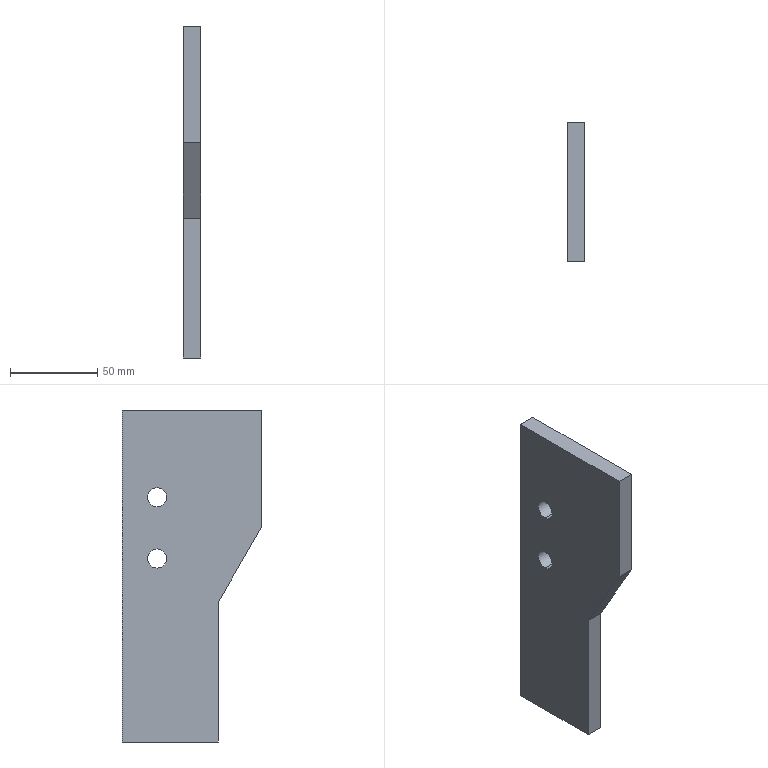Part | STEP file | VD-SYL0380DJ1006_1_5-3_VD-SYL03 | 1 solid | 12 faces | box 10 x 80 x 190 mm | volume 124687 mm3 | plane 8 | cylinder 4 | commonest cylinder face diameters 11 x4
STEP:
#1=CARTESIAN_POINT('',(0.,-20.,-90.5));
#2=VERTEX_POINT('',#1);
#3=CARTESIAN_POINT('',(10.,-20.,-90.5));
#4=VERTEX_POINT('',#3);
#5=CARTESIAN_POINT('',(0.,-20.,-90.5));
#6=DIRECTION('',(1.,0.,0.));
#7=VECTOR('',#6,1000.);
#8=LINE('',#5,#7);
#9=EDGE_CURVE('',#2,#4,#8,.T.);
#10=ORIENTED_EDGE('',*,*,#9,.F.);
#11=CARTESIAN_POINT('',(0.,-20.,-79.5));
#12=VERTEX_POINT('',#11);
#13=CARTESIAN_POINT('',(0.,-20.,-85.));
#14=DIRECTION('',(1.,0.,0.));
#15=DIRECTION('',(0.,0.,1.));
#16=AXIS2_PLACEMENT_3D('',#13,#14,#15);
#17=CIRCLE('',#16,5.5);
#18=EDGE_CURVE('',#12,#2,#17,.T.);
#19=ORIENTED_EDGE('',*,*,#18,.F.);
#20=CARTESIAN_POINT('',(10.,-20.,-79.5));
#21=VERTEX_POINT('',#20);
#22=CARTESIAN_POINT('',(0.,-20.,-79.5));
#23=DIRECTION('',(1.,0.,0.));
#24=VECTOR('',#23,1000.);
#25=LINE('',#22,#24);
#26=EDGE_CURVE('',#12,#21,#25,.T.);
#27=ORIENTED_EDGE('',*,*,#26,.T.);
#28=CARTESIAN_POINT('',(10.,-20.,-85.));
#29=DIRECTION('',(-1.,0.,0.));
#30=DIRECTION('',(0.,0.,-1.));
#31=AXIS2_PLACEMENT_3D('',#28,#29,#30);
#32=CIRCLE('',#31,5.5);
#33=EDGE_CURVE('',#4,#21,#32,.T.);
#34=ORIENTED_EDGE('',*,*,#33,.F.);
#35=EDGE_LOOP('',(#10,#19,#27,#34));
#36=FACE_OUTER_BOUND('',#35,.T.);
#37=CARTESIAN_POINT('',(0.,-20.,-85.));
#38=DIRECTION('',(-1.,0.,0.));
#39=DIRECTION('',(0.,0.,1.));
#40=AXIS2_PLACEMENT_3D('',#37,#38,#39);
#41=CYLINDRICAL_SURFACE('',#40,5.5);
#42=ADVANCED_FACE('',(#36),#41,.F.);
#43=CARTESIAN_POINT('',(10.,-20.,-85.));
#44=DIRECTION('',(-1.,0.,0.));
#45=DIRECTION('',(0.,0.,1.));
#46=AXIS2_PLACEMENT_3D('',#43,#44,#45);
#47=CIRCLE('',#46,5.5);
#48=EDGE_CURVE('',#21,#4,#47,.T.);
#49=ORIENTED_EDGE('',*,*,#48,.F.);
#50=ORIENTED_EDGE('',*,*,#26,.F.);
#51=CARTESIAN_POINT('',(0.,-20.,-85.));
#52=DIRECTION('',(1.,0.,0.));
#53=DIRECTION('',(0.,0.,-1.));
#54=AXIS2_PLACEMENT_3D('',#51,#52,#53);
#55=CIRCLE('',#54,5.5);
#56=EDGE_CURVE('',#2,#12,#55,.T.);
#57=ORIENTED_EDGE('',*,*,#56,.F.);
#58=ORIENTED_EDGE('',*,*,#9,.T.);
#59=EDGE_LOOP('',(#49,#50,#57,#58));
#60=FACE_OUTER_BOUND('',#59,.T.);
#61=CARTESIAN_POINT('',(0.,-20.,-85.));
#62=DIRECTION('',(-1.,0.,0.));
#63=DIRECTION('',(0.,0.,1.));
#64=AXIS2_PLACEMENT_3D('',#61,#62,#63);
#65=CYLINDRICAL_SURFACE('',#64,5.5);
#66=ADVANCED_FACE('',(#60),#65,.F.);
#67=CARTESIAN_POINT('',(0.,-20.,-55.5));
#68=VERTEX_POINT('',#67);
#69=CARTESIAN_POINT('',(10.,-20.,-55.5));
#70=VERTEX_POINT('',#69);
#71=CARTESIAN_POINT('',(0.,-20.,-55.5));
#72=DIRECTION('',(1.,0.,0.));
#73=VECTOR('',#72,1000.);
#74=LINE('',#71,#73);
#75=EDGE_CURVE('',#68,#70,#74,.T.);
#76=ORIENTED_EDGE('',*,*,#75,.F.);
#77=CARTESIAN_POINT('',(0.,-20.,-44.5));
#78=VERTEX_POINT('',#77);
#79=CARTESIAN_POINT('',(0.,-20.,-50.));
#80=DIRECTION('',(1.,0.,0.));
#81=DIRECTION('',(0.,0.,1.));
#82=AXIS2_PLACEMENT_3D('',#79,#80,#81);
#83=CIRCLE('',#82,5.5);
#84=EDGE_CURVE('',#78,#68,#83,.T.);
#85=ORIENTED_EDGE('',*,*,#84,.F.);
#86=CARTESIAN_POINT('',(10.,-20.,-44.5));
#87=VERTEX_POINT('',#86);
#88=CARTESIAN_POINT('',(0.,-20.,-44.5));
#89=DIRECTION('',(1.,0.,0.));
#90=VECTOR('',#89,1000.);
#91=LINE('',#88,#90);
#92=EDGE_CURVE('',#78,#87,#91,.T.);
#93=ORIENTED_EDGE('',*,*,#92,.T.);
#94=CARTESIAN_POINT('',(10.,-20.,-50.));
#95=DIRECTION('',(-1.,0.,0.));
#96=DIRECTION('',(0.,0.,-1.));
#97=AXIS2_PLACEMENT_3D('',#94,#95,#96);
#98=CIRCLE('',#97,5.5);
#99=EDGE_CURVE('',#70,#87,#98,.T.);
#100=ORIENTED_EDGE('',*,*,#99,.F.);
#101=EDGE_LOOP('',(#76,#85,#93,#100));
#102=FACE_OUTER_BOUND('',#101,.T.);
#103=CARTESIAN_POINT('',(0.,-20.,-50.));
#104=DIRECTION('',(-1.,0.,0.));
#105=DIRECTION('',(0.,0.,1.));
#106=AXIS2_PLACEMENT_3D('',#103,#104,#105);
#107=CYLINDRICAL_SURFACE('',#106,5.5);
#108=ADVANCED_FACE('',(#102),#107,.F.);
#109=CARTESIAN_POINT('',(10.,-20.,-50.));
#110=DIRECTION('',(-1.,0.,0.));
#111=DIRECTION('',(0.,0.,1.));
#112=AXIS2_PLACEMENT_3D('',#109,#110,#111);
#113=CIRCLE('',#112,5.5);
#114=EDGE_CURVE('',#87,#70,#113,.T.);
#115=ORIENTED_EDGE('',*,*,#114,.F.);
#116=ORIENTED_EDGE('',*,*,#92,.F.);
#117=CARTESIAN_POINT('',(0.,-20.,-50.));
#118=DIRECTION('',(1.,0.,0.));
#119=DIRECTION('',(0.,0.,-1.));
#120=AXIS2_PLACEMENT_3D('',#117,#118,#119);
#121=CIRCLE('',#120,5.5);
#122=EDGE_CURVE('',#68,#78,#121,.T.);
#123=ORIENTED_EDGE('',*,*,#122,.F.);
#124=ORIENTED_EDGE('',*,*,#75,.T.);
#125=EDGE_LOOP('',(#115,#116,#123,#124));
#126=FACE_OUTER_BOUND('',#125,.T.);
#127=CARTESIAN_POINT('',(0.,-20.,-50.));
#128=DIRECTION('',(-1.,0.,0.));
#129=DIRECTION('',(0.,0.,1.));
#130=AXIS2_PLACEMENT_3D('',#127,#128,#129);
#131=CYLINDRICAL_SURFACE('',#130,5.5);
#132=ADVANCED_FACE('',(#126),#131,.F.);
#133=CARTESIAN_POINT('',(10.,-55.,-110.));
#134=VERTEX_POINT('',#133);
#135=CARTESIAN_POINT('',(10.,-55.,-190.));
#136=VERTEX_POINT('',#135);
#137=CARTESIAN_POINT('',(10.,-55.,-110.));
#138=DIRECTION('',(0.,0.,-1.));
#139=VECTOR('',#138,1000.);
#140=LINE('',#137,#139);
#141=EDGE_CURVE('',#134,#136,#140,.T.);
#142=ORIENTED_EDGE('',*,*,#141,.F.);
#143=CARTESIAN_POINT('',(0.,-55.,-110.));
#144=VERTEX_POINT('',#143);
#145=CARTESIAN_POINT('',(10.,-55.,-110.));
#146=DIRECTION('',(-1.,0.,0.));
#147=VECTOR('',#146,1000.);
#148=LINE('',#145,#147);
#149=EDGE_CURVE('',#134,#144,#148,.T.);
#150=ORIENTED_EDGE('',*,*,#149,.T.);
#151=CARTESIAN_POINT('',(0.,-55.,-190.));
#152=VERTEX_POINT('',#151);
#153=CARTESIAN_POINT('',(0.,-55.,-190.));
#154=DIRECTION('',(0.,0.,1.));
#155=VECTOR('',#154,1000.);
#156=LINE('',#153,#155);
#157=EDGE_CURVE('',#152,#144,#156,.T.);
#158=ORIENTED_EDGE('',*,*,#157,.F.);
#159=CARTESIAN_POINT('',(0.,-55.,-190.));
#160=DIRECTION('',(1.,0.,0.));
#161=VECTOR('',#160,1000.);
#162=LINE('',#159,#161);
#163=EDGE_CURVE('',#152,#136,#162,.T.);
#164=ORIENTED_EDGE('',*,*,#163,.T.);
#165=EDGE_LOOP('',(#142,#150,#158,#164));
#166=FACE_OUTER_BOUND('',#165,.T.);
#167=CARTESIAN_POINT('',(0.,-55.,-110.));
#168=DIRECTION('',(0.,-1.,0.));
#169=DIRECTION('',(0.,0.,-1.));
#170=AXIS2_PLACEMENT_3D('',#167,#168,#169);
#171=PLANE('',#170);
#172=ADVANCED_FACE('',(#166),#171,.T.);
#173=ORIENTED_EDGE('',*,*,#33,.T.);
#174=ORIENTED_EDGE('',*,*,#48,.T.);
#175=EDGE_LOOP('',(#173,#174));
#176=FACE_BOUND('',#175,.T.);
#177=ORIENTED_EDGE('',*,*,#99,.T.);
#178=ORIENTED_EDGE('',*,*,#114,.T.);
#179=EDGE_LOOP('',(#177,#178));
#180=FACE_BOUND('',#179,.T.);
#181=CARTESIAN_POINT('',(10.,0.,-190.));
#182=VERTEX_POINT('',#181);
#183=CARTESIAN_POINT('',(10.,0.,0.));
#184=VERTEX_POINT('',#183);
#185=CARTESIAN_POINT('',(10.,0.,-190.));
#186=DIRECTION('',(0.,0.,1.));
#187=VECTOR('',#186,1000.);
#188=LINE('',#185,#187);
#189=EDGE_CURVE('',#182,#184,#188,.T.);
#190=ORIENTED_EDGE('',*,*,#189,.T.);
#191=CARTESIAN_POINT('',(10.,-80.,0.));
#192=VERTEX_POINT('',#191);
#193=CARTESIAN_POINT('',(10.,0.,0.));
#194=DIRECTION('',(0.,-1.,0.));
#195=VECTOR('',#194,1000.);
#196=LINE('',#193,#195);
#197=EDGE_CURVE('',#184,#192,#196,.T.);
#198=ORIENTED_EDGE('',*,*,#197,.T.);
#199=CARTESIAN_POINT('',(10.,-80.,-66.699));
#200=VERTEX_POINT('',#199);
#201=CARTESIAN_POINT('',(10.,-80.,0.));
#202=DIRECTION('',(0.,0.,-1.));
#203=VECTOR('',#202,1000.);
#204=LINE('',#201,#203);
#205=EDGE_CURVE('',#192,#200,#204,.T.);
#206=ORIENTED_EDGE('',*,*,#205,.T.);
#207=CARTESIAN_POINT('',(10.,-80.,-66.699));
#208=DIRECTION('',(0.,0.5,-0.866));
#209=VECTOR('',#208,1000.);
#210=LINE('',#207,#209);
#211=EDGE_CURVE('',#200,#134,#210,.T.);
#212=ORIENTED_EDGE('',*,*,#211,.T.);
#213=ORIENTED_EDGE('',*,*,#141,.T.);
#214=CARTESIAN_POINT('',(10.,-55.,-190.));
#215=DIRECTION('',(0.,1.,0.));
#216=VECTOR('',#215,1000.);
#217=LINE('',#214,#216);
#218=EDGE_CURVE('',#136,#182,#217,.T.);
#219=ORIENTED_EDGE('',*,*,#218,.T.);
#220=EDGE_LOOP('',(#190,#198,#206,#212,#213,#219));
#221=FACE_OUTER_BOUND('',#220,.T.);
#222=CARTESIAN_POINT('',(10.,0.,0.));
#223=DIRECTION('',(1.,0.,0.));
#224=DIRECTION('',(0.,1.,0.));
#225=AXIS2_PLACEMENT_3D('',#222,#223,#224);
#226=PLANE('',#225);
#227=ADVANCED_FACE('',(#176,#180,#221),#226,.T.);
#228=CARTESIAN_POINT('',(0.,-80.,-66.699));
#229=VERTEX_POINT('',#228);
#230=CARTESIAN_POINT('',(0.,-55.,-110.));
#231=DIRECTION('',(0.,-0.5,0.866));
#232=VECTOR('',#231,1000.);
#233=LINE('',#230,#232);
#234=EDGE_CURVE('',#144,#229,#233,.T.);
#235=ORIENTED_EDGE('',*,*,#234,.F.);
#236=ORIENTED_EDGE('',*,*,#149,.F.);
#237=ORIENTED_EDGE('',*,*,#211,.F.);
#238=CARTESIAN_POINT('',(0.,-80.,-66.699));
#239=DIRECTION('',(1.,0.,0.));
#240=VECTOR('',#239,1000.);
#241=LINE('',#238,#240);
#242=EDGE_CURVE('',#229,#200,#241,.T.);
#243=ORIENTED_EDGE('',*,*,#242,.F.);
#244=EDGE_LOOP('',(#235,#236,#237,#243));
#245=FACE_OUTER_BOUND('',#244,.T.);
#246=CARTESIAN_POINT('',(0.,-80.,-66.699));
#247=DIRECTION('',(0.,-0.866,-0.5));
#248=DIRECTION('',(0.,0.5,-0.866));
#249=AXIS2_PLACEMENT_3D('',#246,#247,#248);
#250=PLANE('',#249);
#251=ADVANCED_FACE('',(#245),#250,.T.);
#252=ORIENTED_EDGE('',*,*,#18,.T.);
#253=ORIENTED_EDGE('',*,*,#56,.T.);
#254=EDGE_LOOP('',(#252,#253));
#255=FACE_BOUND('',#254,.T.);
#256=ORIENTED_EDGE('',*,*,#84,.T.);
#257=ORIENTED_EDGE('',*,*,#122,.T.);
#258=EDGE_LOOP('',(#256,#257));
#259=FACE_BOUND('',#258,.T.);
#260=CARTESIAN_POINT('',(0.,-80.,0.));
#261=VERTEX_POINT('',#260);
#262=CARTESIAN_POINT('',(0.,0.,0.));
#263=VERTEX_POINT('',#262);
#264=CARTESIAN_POINT('',(0.,-80.,0.));
#265=DIRECTION('',(0.,1.,0.));
#266=VECTOR('',#265,1000.);
#267=LINE('',#264,#266);
#268=EDGE_CURVE('',#261,#263,#267,.T.);
#269=ORIENTED_EDGE('',*,*,#268,.T.);
#270=CARTESIAN_POINT('',(0.,0.,-190.));
#271=VERTEX_POINT('',#270);
#272=CARTESIAN_POINT('',(0.,0.,0.));
#273=DIRECTION('',(0.,0.,-1.));
#274=VECTOR('',#273,1000.);
#275=LINE('',#272,#274);
#276=EDGE_CURVE('',#263,#271,#275,.T.);
#277=ORIENTED_EDGE('',*,*,#276,.T.);
#278=CARTESIAN_POINT('',(0.,0.,-190.));
#279=DIRECTION('',(0.,-1.,0.));
#280=VECTOR('',#279,1000.);
#281=LINE('',#278,#280);
#282=EDGE_CURVE('',#271,#152,#281,.T.);
#283=ORIENTED_EDGE('',*,*,#282,.T.);
#284=ORIENTED_EDGE('',*,*,#157,.T.);
#285=ORIENTED_EDGE('',*,*,#234,.T.);
#286=CARTESIAN_POINT('',(0.,-80.,-66.699));
#287=DIRECTION('',(0.,0.,1.));
#288=VECTOR('',#287,1000.);
#289=LINE('',#286,#288);
#290=EDGE_CURVE('',#229,#261,#289,.T.);
#291=ORIENTED_EDGE('',*,*,#290,.T.);
#292=EDGE_LOOP('',(#269,#277,#283,#284,#285,#291));
#293=FACE_OUTER_BOUND('',#292,.T.);
#294=CARTESIAN_POINT('',(0.,0.,0.));
#295=DIRECTION('',(1.,0.,0.));
#296=DIRECTION('',(0.,1.,0.));
#297=AXIS2_PLACEMENT_3D('',#294,#295,#296);
#298=PLANE('',#297);
#299=ADVANCED_FACE('',(#255,#259,#293),#298,.F.);
#300=CARTESIAN_POINT('',(0.,0.,-190.));
#301=DIRECTION('',(1.,0.,0.));
#302=VECTOR('',#301,1000.);
#303=LINE('',#300,#302);
#304=EDGE_CURVE('',#271,#182,#303,.T.);
#305=ORIENTED_EDGE('',*,*,#304,.T.);
#306=ORIENTED_EDGE('',*,*,#218,.F.);
#307=ORIENTED_EDGE('',*,*,#163,.F.);
#308=ORIENTED_EDGE('',*,*,#282,.F.);
#309=EDGE_LOOP('',(#305,#306,#307,#308));
#310=FACE_OUTER_BOUND('',#309,.T.);
#311=CARTESIAN_POINT('',(0.,0.,-190.));
#312=DIRECTION('',(0.,0.,-1.));
#313=DIRECTION('',(0.,-1.,0.));
#314=AXIS2_PLACEMENT_3D('',#311,#312,#313);
#315=PLANE('',#314);
#316=ADVANCED_FACE('',(#310),#315,.T.);
#317=ORIENTED_EDGE('',*,*,#276,.F.);
#318=CARTESIAN_POINT('',(0.,0.,0.));
#319=DIRECTION('',(1.,0.,0.));
#320=VECTOR('',#319,1000.);
#321=LINE('',#318,#320);
#322=EDGE_CURVE('',#263,#184,#321,.T.);
#323=ORIENTED_EDGE('',*,*,#322,.T.);
#324=ORIENTED_EDGE('',*,*,#189,.F.);
#325=ORIENTED_EDGE('',*,*,#304,.F.);
#326=EDGE_LOOP('',(#317,#323,#324,#325));
#327=FACE_OUTER_BOUND('',#326,.T.);
#328=CARTESIAN_POINT('',(0.,0.,-180.));
#329=DIRECTION('',(0.,1.,0.));
#330=DIRECTION('',(1.,0.,0.));
#331=AXIS2_PLACEMENT_3D('',#328,#329,#330);
#332=PLANE('',#331);
#333=ADVANCED_FACE('',(#327),#332,.T.);
#334=ORIENTED_EDGE('',*,*,#268,.F.);
#335=CARTESIAN_POINT('',(0.,-80.,0.));
#336=DIRECTION('',(1.,0.,0.));
#337=VECTOR('',#336,1000.);
#338=LINE('',#335,#337);
#339=EDGE_CURVE('',#261,#192,#338,.T.);
#340=ORIENTED_EDGE('',*,*,#339,.T.);
#341=ORIENTED_EDGE('',*,*,#197,.F.);
#342=ORIENTED_EDGE('',*,*,#322,.F.);
#343=EDGE_LOOP('',(#334,#340,#341,#342));
#344=FACE_OUTER_BOUND('',#343,.T.);
#345=CARTESIAN_POINT('',(0.,0.,0.));
#346=DIRECTION('',(0.,0.,1.));
#347=DIRECTION('',(1.,0.,0.));
#348=AXIS2_PLACEMENT_3D('',#345,#346,#347);
#349=PLANE('',#348);
#350=ADVANCED_FACE('',(#344),#349,.T.);
#351=ORIENTED_EDGE('',*,*,#290,.F.);
#352=ORIENTED_EDGE('',*,*,#242,.T.);
#353=ORIENTED_EDGE('',*,*,#205,.F.);
#354=ORIENTED_EDGE('',*,*,#339,.F.);
#355=EDGE_LOOP('',(#351,#352,#353,#354));
#356=FACE_OUTER_BOUND('',#355,.T.);
#357=CARTESIAN_POINT('',(0.,-80.,0.));
#358=DIRECTION('',(0.,-1.,0.));
#359=DIRECTION('',(0.,0.,-1.));
#360=AXIS2_PLACEMENT_3D('',#357,#358,#359);
#361=PLANE('',#360);
#362=ADVANCED_FACE('',(#356),#361,.T.);
#363=CLOSED_SHELL('',(#42,#66,#108,#132,#172,#227,#251,#299,#316,#333,#350,#362));
#364=MANIFOLD_SOLID_BREP('',#363);
#365=CARTESIAN_POINT('',(0.,0.,0.));
#366=DIRECTION('',(0.,0.,1.));
#367=DIRECTION('',(1.,0.,0.));
#368=AXIS2_PLACEMENT_3D('',#365,#366,#367);
#369=(LENGTH_UNIT()NAMED_UNIT(*)SI_UNIT(.MILLI.,.METRE.));
#370=UNCERTAINTY_MEASURE_WITH_UNIT(LENGTH_MEASURE(0.00001),#369,'','');
#371=(NAMED_UNIT(*)PLANE_ANGLE_UNIT()SI_UNIT($,.RADIAN.));
#372=(NAMED_UNIT(*)SI_UNIT($,.STERADIAN.)SOLID_ANGLE_UNIT());
#373=(GEOMETRIC_REPRESENTATION_CONTEXT(3)GLOBAL_UNCERTAINTY_ASSIGNED_CONTEXT((#370))GLOBAL_UNIT_ASSIGNED_CONTEXT((#369,#371,#372))REPRESENTATION_CONTEXT('',''));
#374=ADVANCED_BREP_SHAPE_REPRESENTATION('',(#364,#368),#373);